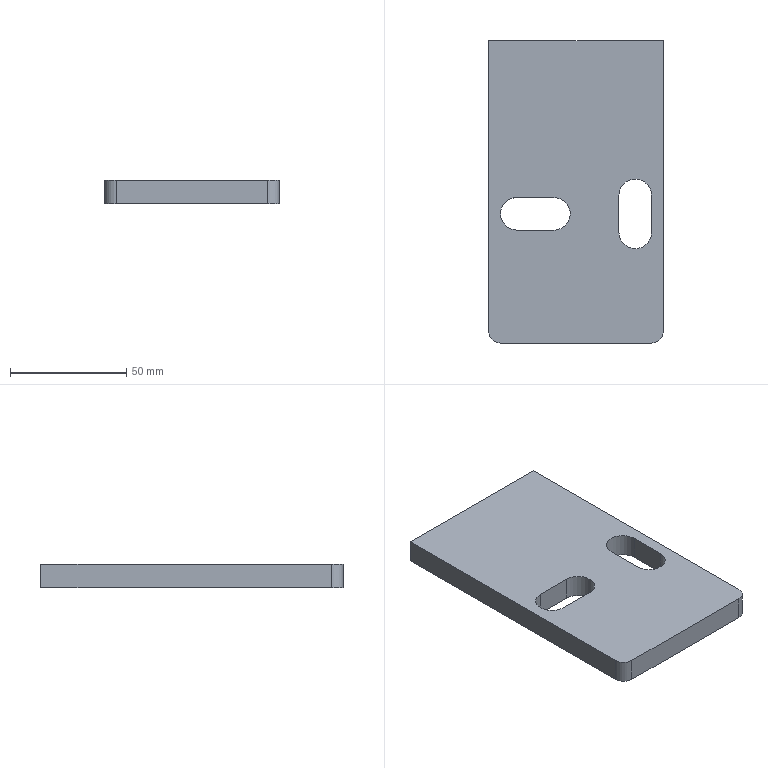Part | SolidWorks | features Extrusion 1 | 1 solid | 18 faces | box 75 x 130 x 10 mm | volume 89834 mm3 | plane 11 | cylinder 7 | commonest cylinder face diameters 14 x5 10 x2
STEP:
#1=CARTESIAN_POINT('',(-25.5,-13.,10.));
#2=VERTEX_POINT('',#1);
#3=CARTESIAN_POINT('',(-32.5,-20.,10.));
#4=VERTEX_POINT('',#3);
#5=CARTESIAN_POINT('',(-25.5,-20.,10.));
#6=DIRECTION('',(0.,0.,1.));
#7=DIRECTION('',(1.,0.,0.));
#8=AXIS2_PLACEMENT_3D('',#5,#6,#7);
#9=CIRCLE('',#8,7.);
#10=EDGE_CURVE('',#2,#4,#9,.T.);
#11=ORIENTED_EDGE('',*,*,#10,.T.);
#12=CARTESIAN_POINT('',(-32.5,-20.,0.));
#13=VERTEX_POINT('',#12);
#14=CARTESIAN_POINT('',(-32.5,-20.,10.));
#15=DIRECTION('',(0.,0.,-1.));
#16=VECTOR('',#15,1000.);
#17=LINE('',#14,#16);
#18=EDGE_CURVE('',#4,#13,#17,.T.);
#19=ORIENTED_EDGE('',*,*,#18,.T.);
#20=CARTESIAN_POINT('',(-25.5,-13.,0.));
#21=VERTEX_POINT('',#20);
#22=CARTESIAN_POINT('',(-25.5,-20.,0.));
#23=DIRECTION('',(0.,0.,1.));
#24=DIRECTION('',(1.,0.,0.));
#25=AXIS2_PLACEMENT_3D('',#22,#23,#24);
#26=CIRCLE('',#25,7.);
#27=EDGE_CURVE('',#21,#13,#26,.T.);
#28=ORIENTED_EDGE('',*,*,#27,.F.);
#29=CARTESIAN_POINT('',(-25.5,-13.,10.));
#30=DIRECTION('',(0.,0.,-1.));
#31=VECTOR('',#30,1000.);
#32=LINE('',#29,#31);
#33=EDGE_CURVE('',#2,#21,#32,.T.);
#34=ORIENTED_EDGE('',*,*,#33,.F.);
#35=EDGE_LOOP('',(#11,#19,#28,#34));
#36=FACE_OUTER_BOUND('',#35,.T.);
#37=CARTESIAN_POINT('',(-25.5,-20.,10.));
#38=DIRECTION('',(0.,0.,-1.));
#39=DIRECTION('',(-1.,0.,0.));
#40=AXIS2_PLACEMENT_3D('',#37,#38,#39);
#41=CYLINDRICAL_SURFACE('',#40,7.);
#42=ADVANCED_FACE('',(#36),#41,.F.);
#43=CARTESIAN_POINT('',(-37.5,54.4,0.));
#44=VERTEX_POINT('',#43);
#45=CARTESIAN_POINT('',(-37.5,-70.6,0.));
#46=VERTEX_POINT('',#45);
#47=CARTESIAN_POINT('',(-37.5,0.,0.));
#48=DIRECTION('',(0.,-1.,0.));
#49=VECTOR('',#48,1000.);
#50=LINE('',#47,#49);
#51=EDGE_CURVE('',#44,#46,#50,.T.);
#52=ORIENTED_EDGE('',*,*,#51,.T.);
#53=CARTESIAN_POINT('',(-37.5,-70.6,10.));
#54=VERTEX_POINT('',#53);
#55=CARTESIAN_POINT('',(-37.5,-70.6,10.));
#56=DIRECTION('',(0.,0.,-1.));
#57=VECTOR('',#56,1000.);
#58=LINE('',#55,#57);
#59=EDGE_CURVE('',#54,#46,#58,.T.);
#60=ORIENTED_EDGE('',*,*,#59,.F.);
#61=CARTESIAN_POINT('',(-37.5,54.4,10.));
#62=VERTEX_POINT('',#61);
#63=CARTESIAN_POINT('',(-37.5,0.,10.));
#64=DIRECTION('',(0.,-1.,0.));
#65=VECTOR('',#64,1000.);
#66=LINE('',#63,#65);
#67=EDGE_CURVE('',#62,#54,#66,.T.);
#68=ORIENTED_EDGE('',*,*,#67,.F.);
#69=CARTESIAN_POINT('',(-37.5,54.4,10.));
#70=DIRECTION('',(0.,0.,-1.));
#71=VECTOR('',#70,1000.);
#72=LINE('',#69,#71);
#73=EDGE_CURVE('',#62,#44,#72,.T.);
#74=ORIENTED_EDGE('',*,*,#73,.T.);
#75=EDGE_LOOP('',(#52,#60,#68,#74));
#76=FACE_OUTER_BOUND('',#75,.T.);
#77=CARTESIAN_POINT('',(-37.5,0.,10.));
#78=DIRECTION('',(1.,0.,0.));
#79=DIRECTION('',(0.,1.,0.));
#80=AXIS2_PLACEMENT_3D('',#77,#78,#79);
#81=PLANE('',#80);
#82=ADVANCED_FACE('',(#76),#81,.F.);
#83=CARTESIAN_POINT('',(-32.5,-75.6,0.));
#84=VERTEX_POINT('',#83);
#85=CARTESIAN_POINT('',(-32.5,-70.6,0.));
#86=DIRECTION('',(0.,0.,1.));
#87=DIRECTION('',(1.,0.,0.));
#88=AXIS2_PLACEMENT_3D('',#85,#86,#87);
#89=CIRCLE('',#88,5.);
#90=EDGE_CURVE('',#46,#84,#89,.T.);
#91=ORIENTED_EDGE('',*,*,#90,.T.);
#92=CARTESIAN_POINT('',(-32.5,-75.6,10.));
#93=VERTEX_POINT('',#92);
#94=CARTESIAN_POINT('',(-32.5,-75.6,10.));
#95=DIRECTION('',(0.,0.,-1.));
#96=VECTOR('',#95,1000.);
#97=LINE('',#94,#96);
#98=EDGE_CURVE('',#93,#84,#97,.T.);
#99=ORIENTED_EDGE('',*,*,#98,.F.);
#100=CARTESIAN_POINT('',(-32.5,-70.6,10.));
#101=DIRECTION('',(0.,0.,1.));
#102=DIRECTION('',(1.,0.,0.));
#103=AXIS2_PLACEMENT_3D('',#100,#101,#102);
#104=CIRCLE('',#103,5.);
#105=EDGE_CURVE('',#54,#93,#104,.T.);
#106=ORIENTED_EDGE('',*,*,#105,.F.);
#107=ORIENTED_EDGE('',*,*,#59,.T.);
#108=EDGE_LOOP('',(#91,#99,#106,#107));
#109=FACE_OUTER_BOUND('',#108,.T.);
#110=CARTESIAN_POINT('',(-32.5,-70.6,10.));
#111=DIRECTION('',(0.,0.,-1.));
#112=DIRECTION('',(-1.,0.,0.));
#113=AXIS2_PLACEMENT_3D('',#110,#111,#112);
#114=CYLINDRICAL_SURFACE('',#113,5.);
#115=ADVANCED_FACE('',(#109),#114,.T.);
#116=CARTESIAN_POINT('',(32.5,-75.6,0.));
#117=VERTEX_POINT('',#116);
#118=CARTESIAN_POINT('',(0.,-75.6,0.));
#119=DIRECTION('',(1.,0.,0.));
#120=VECTOR('',#119,1000.);
#121=LINE('',#118,#120);
#122=EDGE_CURVE('',#84,#117,#121,.T.);
#123=ORIENTED_EDGE('',*,*,#122,.T.);
#124=CARTESIAN_POINT('',(32.5,-75.6,10.));
#125=VERTEX_POINT('',#124);
#126=CARTESIAN_POINT('',(32.5,-75.6,10.));
#127=DIRECTION('',(0.,0.,-1.));
#128=VECTOR('',#127,1000.);
#129=LINE('',#126,#128);
#130=EDGE_CURVE('',#125,#117,#129,.T.);
#131=ORIENTED_EDGE('',*,*,#130,.F.);
#132=CARTESIAN_POINT('',(0.,-75.6,10.));
#133=DIRECTION('',(1.,0.,0.));
#134=VECTOR('',#133,1000.);
#135=LINE('',#132,#134);
#136=EDGE_CURVE('',#93,#125,#135,.T.);
#137=ORIENTED_EDGE('',*,*,#136,.F.);
#138=ORIENTED_EDGE('',*,*,#98,.T.);
#139=EDGE_LOOP('',(#123,#131,#137,#138));
#140=FACE_OUTER_BOUND('',#139,.T.);
#141=CARTESIAN_POINT('',(0.,-75.6,10.));
#142=DIRECTION('',(0.,1.,0.));
#143=DIRECTION('',(-1.,0.,0.));
#144=AXIS2_PLACEMENT_3D('',#141,#142,#143);
#145=PLANE('',#144);
#146=ADVANCED_FACE('',(#140),#145,.F.);
#147=CARTESIAN_POINT('',(37.5,-70.6,0.));
#148=VERTEX_POINT('',#147);
#149=CARTESIAN_POINT('',(32.5,-70.6,0.));
#150=DIRECTION('',(0.,0.,1.));
#151=DIRECTION('',(1.,0.,0.));
#152=AXIS2_PLACEMENT_3D('',#149,#150,#151);
#153=CIRCLE('',#152,5.);
#154=EDGE_CURVE('',#117,#148,#153,.T.);
#155=ORIENTED_EDGE('',*,*,#154,.T.);
#156=CARTESIAN_POINT('',(37.5,-70.6,10.));
#157=VERTEX_POINT('',#156);
#158=CARTESIAN_POINT('',(37.5,-70.6,10.));
#159=DIRECTION('',(0.,0.,-1.));
#160=VECTOR('',#159,1000.);
#161=LINE('',#158,#160);
#162=EDGE_CURVE('',#157,#148,#161,.T.);
#163=ORIENTED_EDGE('',*,*,#162,.F.);
#164=CARTESIAN_POINT('',(32.5,-70.6,10.));
#165=DIRECTION('',(0.,0.,1.));
#166=DIRECTION('',(1.,0.,0.));
#167=AXIS2_PLACEMENT_3D('',#164,#165,#166);
#168=CIRCLE('',#167,5.);
#169=EDGE_CURVE('',#125,#157,#168,.T.);
#170=ORIENTED_EDGE('',*,*,#169,.F.);
#171=ORIENTED_EDGE('',*,*,#130,.T.);
#172=EDGE_LOOP('',(#155,#163,#170,#171));
#173=FACE_OUTER_BOUND('',#172,.T.);
#174=CARTESIAN_POINT('',(32.5,-70.6,10.));
#175=DIRECTION('',(0.,0.,-1.));
#176=DIRECTION('',(-1.,0.,0.));
#177=AXIS2_PLACEMENT_3D('',#174,#175,#176);
#178=CYLINDRICAL_SURFACE('',#177,5.);
#179=ADVANCED_FACE('',(#173),#178,.T.);
#180=CARTESIAN_POINT('',(37.5,54.4,0.));
#181=VERTEX_POINT('',#180);
#182=CARTESIAN_POINT('',(37.5,0.,0.));
#183=DIRECTION('',(0.,-1.,0.));
#184=VECTOR('',#183,1000.);
#185=LINE('',#182,#184);
#186=EDGE_CURVE('',#181,#148,#185,.T.);
#187=ORIENTED_EDGE('',*,*,#186,.F.);
#188=CARTESIAN_POINT('',(37.5,54.4,10.));
#189=VERTEX_POINT('',#188);
#190=CARTESIAN_POINT('',(37.5,54.4,10.));
#191=DIRECTION('',(0.,0.,-1.));
#192=VECTOR('',#191,1000.);
#193=LINE('',#190,#192);
#194=EDGE_CURVE('',#189,#181,#193,.T.);
#195=ORIENTED_EDGE('',*,*,#194,.F.);
#196=CARTESIAN_POINT('',(37.5,0.,10.));
#197=DIRECTION('',(0.,-1.,0.));
#198=VECTOR('',#197,1000.);
#199=LINE('',#196,#198);
#200=EDGE_CURVE('',#189,#157,#199,.T.);
#201=ORIENTED_EDGE('',*,*,#200,.T.);
#202=ORIENTED_EDGE('',*,*,#162,.T.);
#203=EDGE_LOOP('',(#187,#195,#201,#202));
#204=FACE_OUTER_BOUND('',#203,.T.);
#205=CARTESIAN_POINT('',(37.5,0.,10.));
#206=DIRECTION('',(1.,0.,0.));
#207=DIRECTION('',(0.,1.,0.));
#208=AXIS2_PLACEMENT_3D('',#205,#206,#207);
#209=PLANE('',#208);
#210=ADVANCED_FACE('',(#204),#209,.T.);
#211=CARTESIAN_POINT('',(18.5,-28.,0.));
#212=VERTEX_POINT('',#211);
#213=CARTESIAN_POINT('',(32.5,-28.,0.));
#214=VERTEX_POINT('',#213);
#215=CARTESIAN_POINT('',(25.5,-28.,0.));
#216=DIRECTION('',(0.,0.,1.));
#217=DIRECTION('',(1.,0.,0.));
#218=AXIS2_PLACEMENT_3D('',#215,#216,#217);
#219=CIRCLE('',#218,7.);
#220=EDGE_CURVE('',#212,#214,#219,.T.);
#221=ORIENTED_EDGE('',*,*,#220,.F.);
#222=CARTESIAN_POINT('',(18.5,-28.,10.));
#223=VERTEX_POINT('',#222);
#224=CARTESIAN_POINT('',(18.5,-28.,10.));
#225=DIRECTION('',(0.,0.,-1.));
#226=VECTOR('',#225,1000.);
#227=LINE('',#224,#226);
#228=EDGE_CURVE('',#223,#212,#227,.T.);
#229=ORIENTED_EDGE('',*,*,#228,.F.);
#230=CARTESIAN_POINT('',(32.5,-28.,10.));
#231=VERTEX_POINT('',#230);
#232=CARTESIAN_POINT('',(25.5,-28.,10.));
#233=DIRECTION('',(0.,0.,1.));
#234=DIRECTION('',(1.,0.,0.));
#235=AXIS2_PLACEMENT_3D('',#232,#233,#234);
#236=CIRCLE('',#235,7.);
#237=EDGE_CURVE('',#223,#231,#236,.T.);
#238=ORIENTED_EDGE('',*,*,#237,.T.);
#239=CARTESIAN_POINT('',(32.5,-28.,10.));
#240=DIRECTION('',(0.,0.,-1.));
#241=VECTOR('',#240,1000.);
#242=LINE('',#239,#241);
#243=EDGE_CURVE('',#231,#214,#242,.T.);
#244=ORIENTED_EDGE('',*,*,#243,.T.);
#245=EDGE_LOOP('',(#221,#229,#238,#244));
#246=FACE_OUTER_BOUND('',#245,.T.);
#247=CARTESIAN_POINT('',(25.5,-28.,10.));
#248=DIRECTION('',(0.,0.,-1.));
#249=DIRECTION('',(-1.,0.,0.));
#250=AXIS2_PLACEMENT_3D('',#247,#248,#249);
#251=CYLINDRICAL_SURFACE('',#250,7.);
#252=ADVANCED_FACE('',(#246),#251,.F.);
#253=CARTESIAN_POINT('',(18.5,-12.,0.));
#254=VERTEX_POINT('',#253);
#255=CARTESIAN_POINT('',(18.5,0.,0.));
#256=DIRECTION('',(0.,-1.,0.));
#257=VECTOR('',#256,1000.);
#258=LINE('',#255,#257);
#259=EDGE_CURVE('',#254,#212,#258,.T.);
#260=ORIENTED_EDGE('',*,*,#259,.F.);
#261=CARTESIAN_POINT('',(18.5,-12.,10.));
#262=VERTEX_POINT('',#261);
#263=CARTESIAN_POINT('',(18.5,-12.,10.));
#264=DIRECTION('',(0.,0.,-1.));
#265=VECTOR('',#264,1000.);
#266=LINE('',#263,#265);
#267=EDGE_CURVE('',#262,#254,#266,.T.);
#268=ORIENTED_EDGE('',*,*,#267,.F.);
#269=CARTESIAN_POINT('',(18.5,0.,10.));
#270=DIRECTION('',(0.,-1.,0.));
#271=VECTOR('',#270,1000.);
#272=LINE('',#269,#271);
#273=EDGE_CURVE('',#262,#223,#272,.T.);
#274=ORIENTED_EDGE('',*,*,#273,.T.);
#275=ORIENTED_EDGE('',*,*,#228,.T.);
#276=EDGE_LOOP('',(#260,#268,#274,#275));
#277=FACE_OUTER_BOUND('',#276,.T.);
#278=CARTESIAN_POINT('',(18.5,0.,10.));
#279=DIRECTION('',(1.,0.,0.));
#280=DIRECTION('',(0.,0.,-1.));
#281=AXIS2_PLACEMENT_3D('',#278,#279,#280);
#282=PLANE('',#281);
#283=ADVANCED_FACE('',(#277),#282,.T.);
#284=CARTESIAN_POINT('',(32.5,-12.,0.));
#285=VERTEX_POINT('',#284);
#286=CARTESIAN_POINT('',(25.5,-12.,0.));
#287=DIRECTION('',(0.,0.,1.));
#288=DIRECTION('',(1.,0.,0.));
#289=AXIS2_PLACEMENT_3D('',#286,#287,#288);
#290=CIRCLE('',#289,7.);
#291=EDGE_CURVE('',#285,#254,#290,.T.);
#292=ORIENTED_EDGE('',*,*,#291,.F.);
#293=CARTESIAN_POINT('',(32.5,-12.,10.));
#294=VERTEX_POINT('',#293);
#295=CARTESIAN_POINT('',(32.5,-12.,10.));
#296=DIRECTION('',(0.,0.,-1.));
#297=VECTOR('',#296,1000.);
#298=LINE('',#295,#297);
#299=EDGE_CURVE('',#294,#285,#298,.T.);
#300=ORIENTED_EDGE('',*,*,#299,.F.);
#301=CARTESIAN_POINT('',(25.5,-12.,10.));
#302=DIRECTION('',(0.,0.,1.));
#303=DIRECTION('',(1.,0.,0.));
#304=AXIS2_PLACEMENT_3D('',#301,#302,#303);
#305=CIRCLE('',#304,7.);
#306=EDGE_CURVE('',#294,#262,#305,.T.);
#307=ORIENTED_EDGE('',*,*,#306,.T.);
#308=ORIENTED_EDGE('',*,*,#267,.T.);
#309=EDGE_LOOP('',(#292,#300,#307,#308));
#310=FACE_OUTER_BOUND('',#309,.T.);
#311=CARTESIAN_POINT('',(25.5,-12.,10.));
#312=DIRECTION('',(0.,0.,-1.));
#313=DIRECTION('',(-1.,0.,0.));
#314=AXIS2_PLACEMENT_3D('',#311,#312,#313);
#315=CYLINDRICAL_SURFACE('',#314,7.);
#316=ADVANCED_FACE('',(#310),#315,.F.);
#317=CARTESIAN_POINT('',(-9.035,-27.,0.));
#318=VERTEX_POINT('',#317);
#319=CARTESIAN_POINT('',(-9.029,-26.984,0.));
#320=VERTEX_POINT('',#319);
#321=CARTESIAN_POINT('',(0.,0.,0.));
#322=DIRECTION('',(0.3173,0.9483,0.));
#323=VECTOR('',#322,1000.);
#324=LINE('',#321,#323);
#325=EDGE_CURVE('',#318,#320,#324,.T.);
#326=ORIENTED_EDGE('',*,*,#325,.F.);
#327=CARTESIAN_POINT('',(-9.035,-27.,10.));
#328=VERTEX_POINT('',#327);
#329=CARTESIAN_POINT('',(-9.035,-27.,10.));
#330=DIRECTION('',(0.,0.,-1.));
#331=VECTOR('',#330,1000.);
#332=LINE('',#329,#331);
#333=EDGE_CURVE('',#328,#318,#332,.T.);
#334=ORIENTED_EDGE('',*,*,#333,.F.);
#335=CARTESIAN_POINT('',(-9.029,-26.984,10.));
#336=VERTEX_POINT('',#335);
#337=CARTESIAN_POINT('',(0.,0.,10.));
#338=DIRECTION('',(0.3173,0.9483,0.));
#339=VECTOR('',#338,1000.);
#340=LINE('',#337,#339);
#341=EDGE_CURVE('',#328,#336,#340,.T.);
#342=ORIENTED_EDGE('',*,*,#341,.T.);
#343=CARTESIAN_POINT('',(-9.029,-26.984,10.));
#344=DIRECTION('',(0.,0.,-1.));
#345=VECTOR('',#344,1000.);
#346=LINE('',#343,#345);
#347=EDGE_CURVE('',#336,#320,#346,.T.);
#348=ORIENTED_EDGE('',*,*,#347,.T.);
#349=EDGE_LOOP('',(#326,#334,#342,#348));
#350=FACE_OUTER_BOUND('',#349,.T.);
#351=CARTESIAN_POINT('',(0.,0.,10.));
#352=DIRECTION('',(-0.9483,0.3173,0.));
#353=DIRECTION('',(-0.3173,-0.9483,0.));
#354=AXIS2_PLACEMENT_3D('',#351,#352,#353);
#355=PLANE('',#354);
#356=ADVANCED_FACE('',(#350),#355,.T.);
#357=CARTESIAN_POINT('',(-25.5,-27.,0.));
#358=VERTEX_POINT('',#357);
#359=CARTESIAN_POINT('',(0.,-27.,0.));
#360=DIRECTION('',(1.,0.,0.));
#361=VECTOR('',#360,1000.);
#362=LINE('',#359,#361);
#363=EDGE_CURVE('',#358,#318,#362,.T.);
#364=ORIENTED_EDGE('',*,*,#363,.F.);
#365=CARTESIAN_POINT('',(-25.5,-27.,10.));
#366=VERTEX_POINT('',#365);
#367=CARTESIAN_POINT('',(-25.5,-27.,10.));
#368=DIRECTION('',(0.,0.,-1.));
#369=VECTOR('',#368,1000.);
#370=LINE('',#367,#369);
#371=EDGE_CURVE('',#366,#358,#370,.T.);
#372=ORIENTED_EDGE('',*,*,#371,.F.);
#373=CARTESIAN_POINT('',(0.,-27.,10.));
#374=DIRECTION('',(1.,0.,0.));
#375=VECTOR('',#374,1000.);
#376=LINE('',#373,#375);
#377=EDGE_CURVE('',#366,#328,#376,.T.);
#378=ORIENTED_EDGE('',*,*,#377,.T.);
#379=ORIENTED_EDGE('',*,*,#333,.T.);
#380=EDGE_LOOP('',(#364,#372,#378,#379));
#381=FACE_OUTER_BOUND('',#380,.T.);
#382=CARTESIAN_POINT('',(0.,-27.,10.));
#383=DIRECTION('',(0.,1.,0.));
#384=DIRECTION('',(0.,0.,1.));
#385=AXIS2_PLACEMENT_3D('',#382,#383,#384);
#386=PLANE('',#385);
#387=ADVANCED_FACE('',(#381),#386,.T.);
#388=ORIENTED_EDGE('',*,*,#18,.F.);
#389=CARTESIAN_POINT('',(-25.5,-20.,10.));
#390=DIRECTION('',(0.,0.,1.));
#391=DIRECTION('',(1.,0.,0.));
#392=AXIS2_PLACEMENT_3D('',#389,#390,#391);
#393=CIRCLE('',#392,7.);
#394=EDGE_CURVE('',#4,#366,#393,.T.);
#395=ORIENTED_EDGE('',*,*,#394,.T.);
#396=ORIENTED_EDGE('',*,*,#371,.T.);
#397=CARTESIAN_POINT('',(-25.5,-20.,0.));
#398=DIRECTION('',(0.,0.,1.));
#399=DIRECTION('',(1.,0.,0.));
#400=AXIS2_PLACEMENT_3D('',#397,#398,#399);
#401=CIRCLE('',#400,7.);
#402=EDGE_CURVE('',#13,#358,#401,.T.);
#403=ORIENTED_EDGE('',*,*,#402,.F.);
#404=EDGE_LOOP('',(#388,#395,#396,#403));
#405=FACE_OUTER_BOUND('',#404,.T.);
#406=CARTESIAN_POINT('',(-25.5,-20.,10.));
#407=DIRECTION('',(0.,0.,-1.));
#408=DIRECTION('',(-1.,0.,0.));
#409=AXIS2_PLACEMENT_3D('',#406,#407,#408);
#410=CYLINDRICAL_SURFACE('',#409,7.);
#411=ADVANCED_FACE('',(#405),#410,.F.);
#412=CARTESIAN_POINT('',(-9.5,-13.,0.));
#413=VERTEX_POINT('',#412);
#414=CARTESIAN_POINT('',(0.,-13.,0.));
#415=DIRECTION('',(1.,0.,0.));
#416=VECTOR('',#415,1000.);
#417=LINE('',#414,#416);
#418=EDGE_CURVE('',#21,#413,#417,.T.);
#419=ORIENTED_EDGE('',*,*,#418,.T.);
#420=CARTESIAN_POINT('',(-9.5,-13.,10.));
#421=VERTEX_POINT('',#420);
#422=CARTESIAN_POINT('',(-9.5,-13.,10.));
#423=DIRECTION('',(0.,0.,-1.));
#424=VECTOR('',#423,1000.);
#425=LINE('',#422,#424);
#426=EDGE_CURVE('',#421,#413,#425,.T.);
#427=ORIENTED_EDGE('',*,*,#426,.F.);
#428=CARTESIAN_POINT('',(0.,-13.,10.));
#429=DIRECTION('',(1.,0.,0.));
#430=VECTOR('',#429,1000.);
#431=LINE('',#428,#430);
#432=EDGE_CURVE('',#2,#421,#431,.T.);
#433=ORIENTED_EDGE('',*,*,#432,.F.);
#434=ORIENTED_EDGE('',*,*,#33,.T.);
#435=EDGE_LOOP('',(#419,#427,#433,#434));
#436=FACE_OUTER_BOUND('',#435,.T.);
#437=CARTESIAN_POINT('',(0.,-13.,10.));
#438=DIRECTION('',(0.,1.,0.));
#439=DIRECTION('',(0.,0.,1.));
#440=AXIS2_PLACEMENT_3D('',#437,#438,#439);
#441=PLANE('',#440);
#442=ADVANCED_FACE('',(#436),#441,.F.);
#443=CARTESIAN_POINT('',(32.5,0.,0.));
#444=DIRECTION('',(0.,-1.,0.));
#445=VECTOR('',#444,1000.);
#446=LINE('',#443,#445);
#447=EDGE_CURVE('',#285,#214,#446,.T.);
#448=ORIENTED_EDGE('',*,*,#447,.T.);
#449=ORIENTED_EDGE('',*,*,#243,.F.);
#450=CARTESIAN_POINT('',(32.5,0.,10.));
#451=DIRECTION('',(0.,-1.,0.));
#452=VECTOR('',#451,1000.);
#453=LINE('',#450,#452);
#454=EDGE_CURVE('',#294,#231,#453,.T.);
#455=ORIENTED_EDGE('',*,*,#454,.F.);
#456=ORIENTED_EDGE('',*,*,#299,.T.);
#457=EDGE_LOOP('',(#448,#449,#455,#456));
#458=FACE_OUTER_BOUND('',#457,.T.);
#459=CARTESIAN_POINT('',(32.5,0.,10.));
#460=DIRECTION('',(1.,0.,0.));
#461=DIRECTION('',(0.,0.,-1.));
#462=AXIS2_PLACEMENT_3D('',#459,#460,#461);
#463=PLANE('',#462);
#464=ADVANCED_FACE('',(#458),#463,.F.);
#465=CARTESIAN_POINT('',(-9.5,-20.,0.));
#466=DIRECTION('',(0.,0.,1.));
#467=DIRECTION('',(1.,0.,0.));
#468=AXIS2_PLACEMENT_3D('',#465,#466,#467);
#469=CIRCLE('',#468,7.);
#470=EDGE_CURVE('',#320,#413,#469,.T.);
#471=ORIENTED_EDGE('',*,*,#470,.F.);
#472=ORIENTED_EDGE('',*,*,#347,.F.);
#473=CARTESIAN_POINT('',(-9.5,-20.,10.));
#474=DIRECTION('',(0.,0.,1.));
#475=DIRECTION('',(1.,0.,0.));
#476=AXIS2_PLACEMENT_3D('',#473,#474,#475);
#477=CIRCLE('',#476,7.);
#478=EDGE_CURVE('',#336,#421,#477,.T.);
#479=ORIENTED_EDGE('',*,*,#478,.T.);
#480=ORIENTED_EDGE('',*,*,#426,.T.);
#481=EDGE_LOOP('',(#471,#472,#479,#480));
#482=FACE_OUTER_BOUND('',#481,.T.);
#483=CARTESIAN_POINT('',(-9.5,-20.,10.));
#484=DIRECTION('',(0.,0.,-1.));
#485=DIRECTION('',(-1.,0.,0.));
#486=AXIS2_PLACEMENT_3D('',#483,#484,#485);
#487=CYLINDRICAL_SURFACE('',#486,7.);
#488=ADVANCED_FACE('',(#482),#487,.F.);
#489=CARTESIAN_POINT('',(0.,54.4,0.));
#490=DIRECTION('',(1.,0.,0.));
#491=VECTOR('',#490,1000.);
#492=LINE('',#489,#491);
#493=EDGE_CURVE('',#44,#181,#492,.T.);
#494=ORIENTED_EDGE('',*,*,#493,.F.);
#495=ORIENTED_EDGE('',*,*,#73,.F.);
#496=CARTESIAN_POINT('',(0.,54.4,10.));
#497=DIRECTION('',(1.,0.,0.));
#498=VECTOR('',#497,1000.);
#499=LINE('',#496,#498);
#500=EDGE_CURVE('',#62,#189,#499,.T.);
#501=ORIENTED_EDGE('',*,*,#500,.T.);
#502=ORIENTED_EDGE('',*,*,#194,.T.);
#503=EDGE_LOOP('',(#494,#495,#501,#502));
#504=FACE_OUTER_BOUND('',#503,.T.);
#505=CARTESIAN_POINT('',(0.,54.4,10.));
#506=DIRECTION('',(0.,1.,0.));
#507=DIRECTION('',(0.,0.,1.));
#508=AXIS2_PLACEMENT_3D('',#505,#506,#507);
#509=PLANE('',#508);
#510=ADVANCED_FACE('',(#504),#509,.T.);
#511=ORIENTED_EDGE('',*,*,#341,.F.);
#512=ORIENTED_EDGE('',*,*,#377,.F.);
#513=ORIENTED_EDGE('',*,*,#394,.F.);
#514=ORIENTED_EDGE('',*,*,#10,.F.);
#515=ORIENTED_EDGE('',*,*,#432,.T.);
#516=ORIENTED_EDGE('',*,*,#478,.F.);
#517=EDGE_LOOP('',(#511,#512,#513,#514,#515,#516));
#518=FACE_BOUND('',#517,.T.);
#519=ORIENTED_EDGE('',*,*,#237,.F.);
#520=ORIENTED_EDGE('',*,*,#273,.F.);
#521=ORIENTED_EDGE('',*,*,#306,.F.);
#522=ORIENTED_EDGE('',*,*,#454,.T.);
#523=EDGE_LOOP('',(#519,#520,#521,#522));
#524=FACE_BOUND('',#523,.T.);
#525=ORIENTED_EDGE('',*,*,#67,.T.);
#526=ORIENTED_EDGE('',*,*,#105,.T.);
#527=ORIENTED_EDGE('',*,*,#136,.T.);
#528=ORIENTED_EDGE('',*,*,#169,.T.);
#529=ORIENTED_EDGE('',*,*,#200,.F.);
#530=ORIENTED_EDGE('',*,*,#500,.F.);
#531=EDGE_LOOP('',(#525,#526,#527,#528,#529,#530));
#532=FACE_OUTER_BOUND('',#531,.T.);
#533=CARTESIAN_POINT('',(0.,0.,10.));
#534=DIRECTION('',(0.,0.,1.));
#535=DIRECTION('',(1.,0.,0.));
#536=AXIS2_PLACEMENT_3D('',#533,#534,#535);
#537=PLANE('',#536);
#538=ADVANCED_FACE('',(#518,#524,#532),#537,.T.);
#539=ORIENTED_EDGE('',*,*,#325,.T.);
#540=ORIENTED_EDGE('',*,*,#470,.T.);
#541=ORIENTED_EDGE('',*,*,#418,.F.);
#542=ORIENTED_EDGE('',*,*,#27,.T.);
#543=ORIENTED_EDGE('',*,*,#402,.T.);
#544=ORIENTED_EDGE('',*,*,#363,.T.);
#545=EDGE_LOOP('',(#539,#540,#541,#542,#543,#544));
#546=FACE_BOUND('',#545,.T.);
#547=ORIENTED_EDGE('',*,*,#220,.T.);
#548=ORIENTED_EDGE('',*,*,#447,.F.);
#549=ORIENTED_EDGE('',*,*,#291,.T.);
#550=ORIENTED_EDGE('',*,*,#259,.T.);
#551=EDGE_LOOP('',(#547,#548,#549,#550));
#552=FACE_BOUND('',#551,.T.);
#553=ORIENTED_EDGE('',*,*,#51,.F.);
#554=ORIENTED_EDGE('',*,*,#493,.T.);
#555=ORIENTED_EDGE('',*,*,#186,.T.);
#556=ORIENTED_EDGE('',*,*,#154,.F.);
#557=ORIENTED_EDGE('',*,*,#122,.F.);
#558=ORIENTED_EDGE('',*,*,#90,.F.);
#559=EDGE_LOOP('',(#553,#554,#555,#556,#557,#558));
#560=FACE_OUTER_BOUND('',#559,.T.);
#561=CARTESIAN_POINT('',(0.,0.,0.));
#562=DIRECTION('',(0.,0.,1.));
#563=DIRECTION('',(1.,0.,0.));
#564=AXIS2_PLACEMENT_3D('',#561,#562,#563);
#565=PLANE('',#564);
#566=ADVANCED_FACE('',(#546,#552,#560),#565,.F.);
#567=CLOSED_SHELL('',(#42,#82,#115,#146,#179,#210,#252,#283,#316,#356,#387,#411,#442,#464,#488,#510,#538,#566));
#568=MANIFOLD_SOLID_BREP('',#567);
#569=CARTESIAN_POINT('',(0.,0.,0.));
#570=DIRECTION('',(0.,0.,1.));
#571=DIRECTION('',(1.,0.,0.));
#572=AXIS2_PLACEMENT_3D('',#569,#570,#571);
#573=(LENGTH_UNIT()NAMED_UNIT(*)SI_UNIT(.MILLI.,.METRE.));
#574=UNCERTAINTY_MEASURE_WITH_UNIT(LENGTH_MEASURE(0.00001),#573,'','');
#575=(NAMED_UNIT(*)PLANE_ANGLE_UNIT()SI_UNIT($,.RADIAN.));
#576=(NAMED_UNIT(*)SI_UNIT($,.STERADIAN.)SOLID_ANGLE_UNIT());
#577=(GEOMETRIC_REPRESENTATION_CONTEXT(3)GLOBAL_UNCERTAINTY_ASSIGNED_CONTEXT((#574))GLOBAL_UNIT_ASSIGNED_CONTEXT((#573,#575,#576))REPRESENTATION_CONTEXT('',''));
#578=ADVANCED_BREP_SHAPE_REPRESENTATION('',(#568,#572),#577);